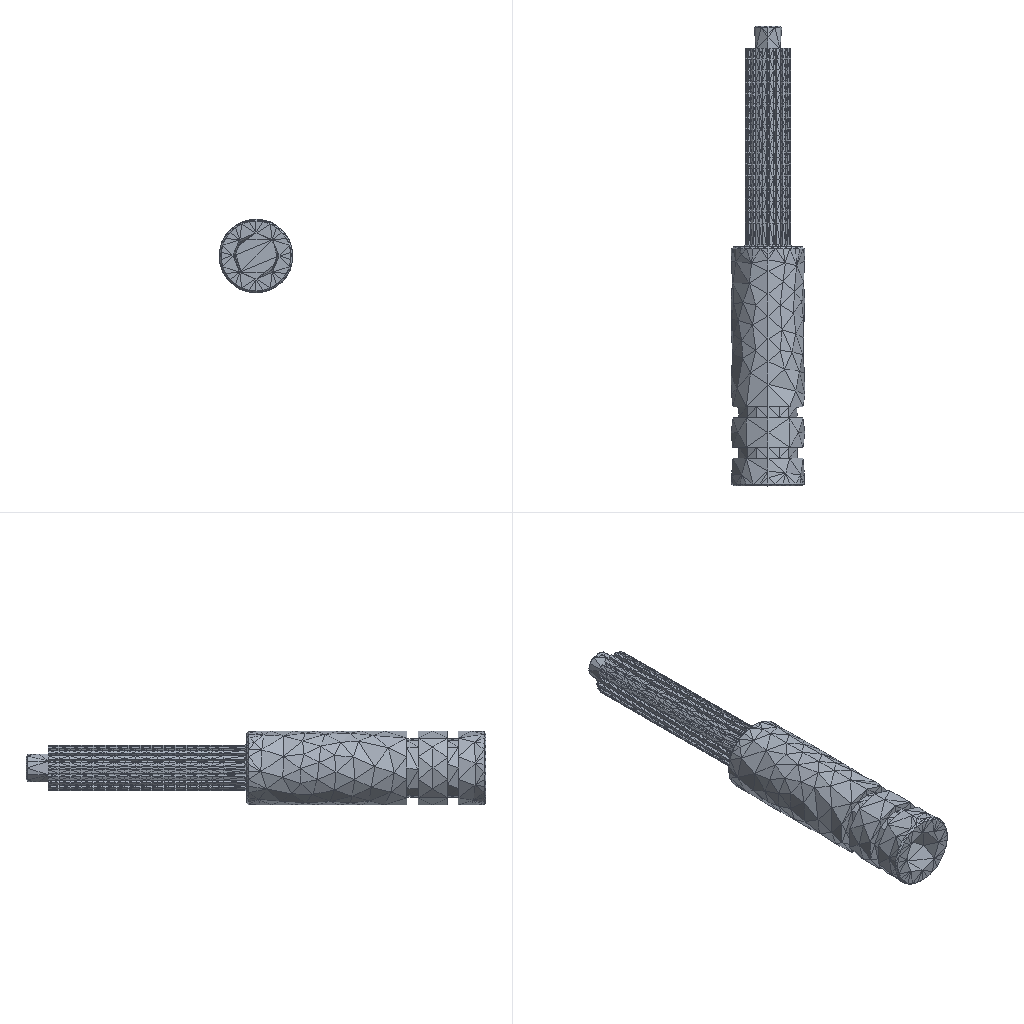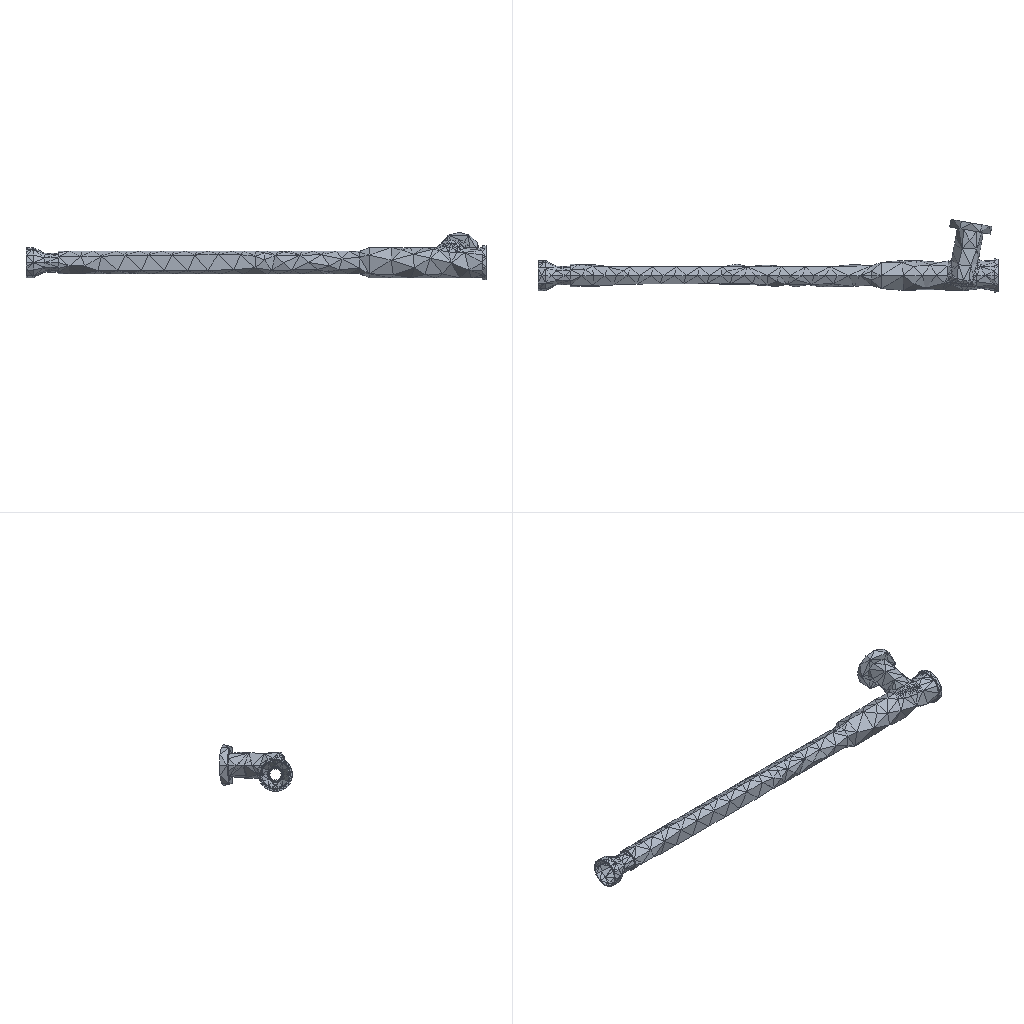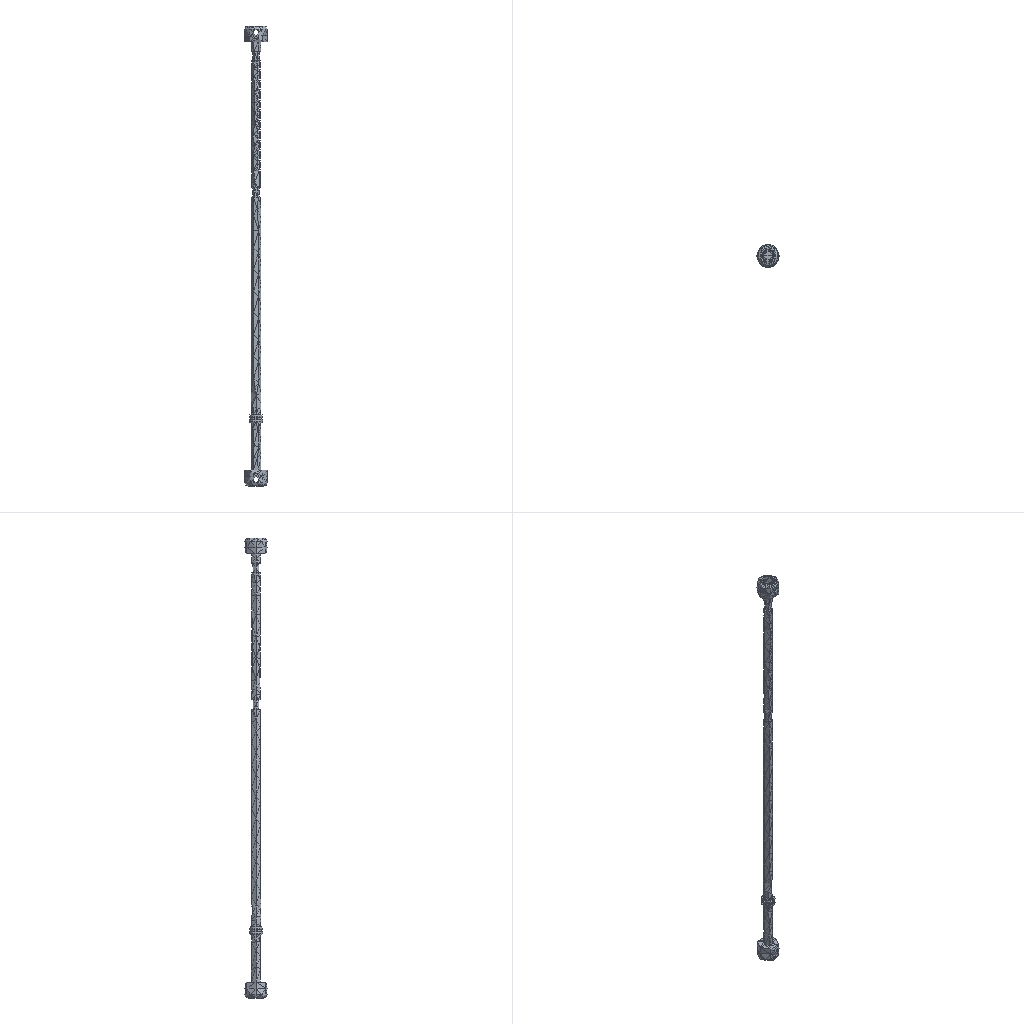Simulation study | ansys workbench
Set-up summary:
category,name,step,type,value,unit,region
solver,ansys_mapdl
solver,version,,,22.1
solver,version,,,22.1
solver,version,,,22.1
solver,version,,,22.1
solver,version,,,22.1
solver,version,,,22.1
solver,version,,,22.1
solver,version,,,22.1
units,MPA,,stated
analysis,deck1,,static,static
load_step,requested,,,1
analysis,nlgeom,,,False
mesh,nodes,,,7630
mesh,elements,,,3798
element_type,ANSYS 187 (type 1),,solid,3600
element_type,ANSYS 154 (type 2),,surface,198
load,load commands in deck,,count,3
bc,support commands in deck,,count,1
named_set,_FIXEDSU,,component
named_set,______,,component
analysis,deck2,,static,static
load_step,requested,,,1
analysis,nlgeom,,,False
mesh,nodes,,,5759
mesh,elements,,,3600
element_type,ANSYS 187 (type 1),,solid,2984
element_type,ANSYS 174 (type 2),,contact,616
element_type,ANSYS 170 (type 3),,target,0
load,load commands in deck,,count,3
bc,support commands in deck,,count,1
named_set,_FIXEDSU,,component
analysis,deck3,,static,static
load_step,requested,,,1
analysis,nlgeom,,,False
mesh,nodes,,,14915
mesh,elements,,,8476
element_type,ANSYS 187 (type 1),,solid,3773
element_type,ANSYS 187 (type 2),,solid,3597
element_type,ANSYS 174 (type 3),,contact,110
element_type,ANSYS 170 (type 4),,target,110
element_type,ANSYS 174 (type 5),,contact,886
element_type,ANSYS 170 (type 6),,target,0
load,load commands in deck,,count,3
bc,support commands in deck,,count,1
named_set,_FIXEDSU,,component
named_set,______,,component
analysis,deck4,,modal,modal
load_step,requested,,,1
analysis,nlgeom,,,False
mesh,nodes,,,13545
mesh,elements,,,7138
element_type,ANSYS 187 (type 1),,solid,7138
load,load commands in deck,,count,0
bc,support commands in deck,,count,0
named_set,______,,component
analysis,deck5,,modal,modal
load_step,requested,,,1
analysis,nlgeom,,,False
mesh,nodes,,,7630
mesh,elements,,,3600
element_type,ANSYS 187 (type 1),,solid,3600
load,load commands in deck,,count,0
bc,support commands in deck,,count,0
named_set,______,,component
analysis,deck6,,modal,modal
load_step,requested,,,1
analysis,nlgeom,,,False
mesh,nodes,,,5759
mesh,elements,,,2984
element_type,ANSYS 187 (type 1),,solid,2984
load,load commands in deck,,count,0
bc,support commands in deck,,count,0
analysis,deck7,,modal,modal
load_step,requested,,,1
analysis,nlgeom,,,False
mesh,nodes,,,14915
mesh,elements,,,7590
element_type,ANSYS 187 (type 1),,solid,3773
element_type,ANSYS 187 (type 2),,solid,3597
element_type,ANSYS 174 (type 3),,contact,110
element_type,ANSYS 170 (type 4),,target,110
load,load commands in deck,,count,0
bc,support commands in deck,,count,0
named_set,______,,component
analysis,deck8,,static,static
load_step,requested,,,1
analysis,nlgeom,,,False
mesh,nodes,,,13545
mesh,elements,,,8604
element_type,ANSYS 187 (type 1),,solid,7138
element_type,ANSYS 174 (type 2),,contact,1466
element_type,ANSYS 170 (type 3),,target,0
load,load commands in deck,,count,3
bc,support commands in deck,,count,1
named_set,_FIXEDSU,,component
named_set,______,,component
material,1,,in results
material,1,,in results
material,1,,in results
material,2,,in results
material,1,,in results
material,1,,in results
material,1,,in results
material,1,,in results
material,2,,in results
material,1,,in results
check,setup vs results,,match,198 surface effect element(s) are not in the reader's mesh and were not compared
check,setup vs results,,match,results also hold 0 node(s) and 1 element(s) the deck makes with ['EN']; those were not compared; 1 node(s) the solver created internally for pilot nodes (ansys-fenxi-2/ansys转向器有限元分析/111111_files/dp0/SYS-2/MECH/solve.out) are in the results only
check,setup vs results,,match,results also hold 0 node(s) and 1 element(s) the deck makes with ['EN']; those were not compared; 1 node(s) the solver created internally for pilot nodes (ansys-fenxi-2/ansys转向器有限元分析/111111_files/dp0/SYS-3/MECH/solve.out) are in the results only
check,setup vs results,,match,1 setup node(s) no element uses are not in the results (e.g. [13545])
check,setup vs results,,match
check,setup vs results,,match,1 setup node(s) no element uses are not in the results (e.g. [5759])
check,setup vs results,,match,1 setup node(s) no element uses are not in the results (e.g. [14915])
check,setup vs results,,match,results also hold 0 node(s) and 1 element(s) the deck makes with ['EN']; those were not compared; 1 node(s) the solver created internally for pilot nodes (ansys-fenxi-2/ansys转向器有限元分析/111111_files/dp0/SYS/MECH/solve.out) are in the results only
Results summary:
result,analysis,,,static
result,last_loadstep,,,1
result,primary field,,,displacement
result,reaction total,1,FX,-0.0,N
result,reaction total,1,FY,0.0,N
result,reaction total,1,FZ,-5000.0,N
result,mass,,,0.008928,"NMM: mm, ton, N, s, mV, mA, degC"
result,analysis,,,static
result,last_loadstep,,,1
result,primary field,,,displacement
result,reaction total,1,FX,0.0,N
result,reaction total,1,FY,-0.0,N
result,reaction total,1,FZ,-0.0,N
result,mass,,,0.01972,"NMM: mm, ton, N, s, mV, mA, degC"
result,analysis,,,static
result,last_loadstep,,,1
result,primary field,,,displacement
result,reaction total,1,FX,-1e-06,N
result,reaction total,1,FY,-1e-06,N
result,reaction total,1,FZ,-0.0,N
result,mass,,,0.01032,"NMM: mm, ton, N, s, mV, mA, degC"
result,analysis,,,modal
result,last_loadstep,,,1
result,primary field,,,displacement
result,analysis,,,modal
result,last_loadstep,,,1
result,primary field,,,displacement
result,analysis,,,modal
result,last_loadstep,,,1
result,primary field,,,displacement
result,analysis,,,modal
result,last_loadstep,,,1
result,primary field,,,displacement
result,analysis,,,static
result,last_loadstep,,,1
result,primary field,,,displacement
result,reaction total,1,FX,0.000167,N
result,reaction total,1,FY,-0.000187,N
result,reaction total,1,FZ,0.000122,N
result,mass,,,0.001393,"NMM: mm, ton, N, s, mV, mA, degC"